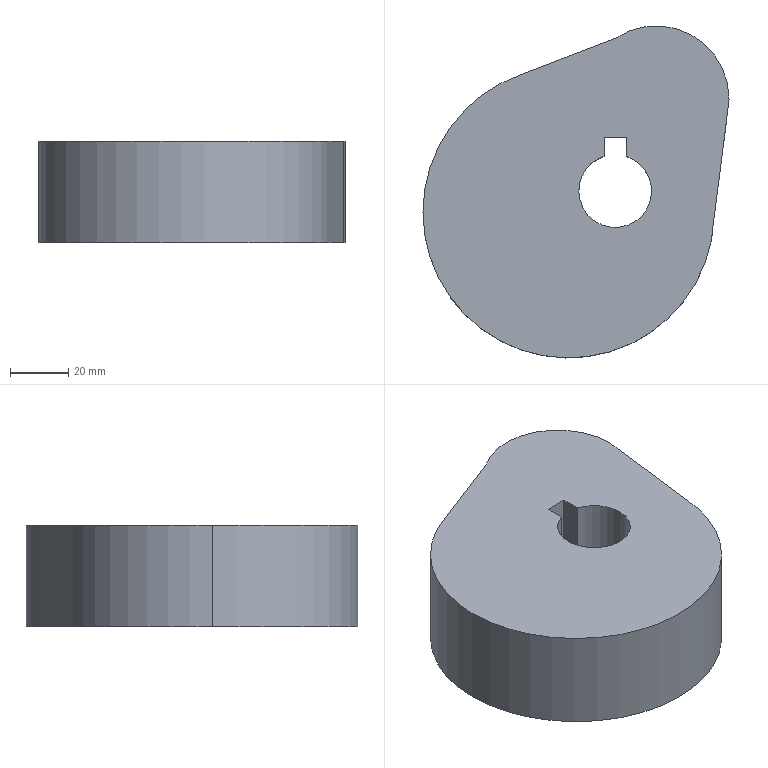Part | STEP file | Disc cam | 1 solid | 13 faces | box 105.129 x 114.018 x 35 mm | volume 298782 mm3 | plane 7 | cylinder 6 | commonest cylinder face diameters 25 x3 100 x2 50 x1
STEP:
#1=CARTESIAN_POINT('',(0.,0.,0.));
#2=DIRECTION('',(0.,0.,1.));
#3=DIRECTION('',(1.,0.,0.));
#4=AXIS2_PLACEMENT_3D('',#1,#2,#3);
#5=CARTESIAN_POINT('',(-6.022,55.403,0.));
#6=VERTEX_POINT('',#5);
#7=CARTESIAN_POINT('',(-6.022,55.403,35.));
#8=VERTEX_POINT('',#7);
#9=CARTESIAN_POINT('',(-6.022,55.403,-109.18));
#10=DIRECTION('',(0.,0.,1.));
#11=VECTOR('',#10,1.);
#12=LINE('',#9,#11);
#13=CARTESIAN_POINT('',(-18.522,55.403,-109.18));
#14=DIRECTION('',(0.,0.,1.));
#15=DIRECTION('',(1.,0.,0.));
#16=AXIS2_PLACEMENT_3D('',#13,#14,#15);
#17=CYLINDRICAL_SURFACE('',#16,12.5);
#18=CARTESIAN_POINT('',(6.283,0.));
#19=DIRECTION('',(0.,1.));
#20=VECTOR('',#19,1.);
#21=LINE('',#18,#20);
#22=(GEOMETRIC_REPRESENTATION_CONTEXT(2)PARAMETRIC_REPRESENTATION_CONTEXT()REPRESENTATION_CONTEXT('',''));
#23=DEFINITIONAL_REPRESENTATION('',(#21),#22);
#24=PCURVE('',#17,#23);
#25=CARTESIAN_POINT('',(-18.522,55.403,-109.18));
#26=DIRECTION('',(0.,0.,1.));
#27=DIRECTION('',(1.,0.,0.));
#28=AXIS2_PLACEMENT_3D('',#25,#26,#27);
#29=CYLINDRICAL_SURFACE('',#28,12.5);
#30=CARTESIAN_POINT('',(0.,0.));
#31=DIRECTION('',(0.,1.));
#32=VECTOR('',#31,1.);
#33=LINE('',#30,#32);
#34=(GEOMETRIC_REPRESENTATION_CONTEXT(2)PARAMETRIC_REPRESENTATION_CONTEXT()REPRESENTATION_CONTEXT('',''));
#35=DEFINITIONAL_REPRESENTATION('',(#33),#34);
#36=PCURVE('',#29,#35);
#37=SURFACE_CURVE('',#12,(#24,#36),.PCURVE_S1.);
#38=EDGE_CURVE('',#6,#8,#37,.T.);
#39=ORIENTED_EDGE('',*,*,#38,.T.);
#40=CARTESIAN_POINT('',(-31.022,55.403,35.));
#41=VERTEX_POINT('',#40);
#42=CARTESIAN_POINT('',(-18.522,55.403,35.));
#43=DIRECTION('',(0.,0.,1.));
#44=DIRECTION('',(1.,0.,0.));
#45=AXIS2_PLACEMENT_3D('',#42,#43,#44);
#46=CIRCLE('',#45,12.5);
#47=CARTESIAN_POINT('',(0.,144.18));
#48=DIRECTION('',(1.,0.));
#49=VECTOR('',#48,1.);
#50=LINE('',#47,#49);
#51=(GEOMETRIC_REPRESENTATION_CONTEXT(2)PARAMETRIC_REPRESENTATION_CONTEXT()REPRESENTATION_CONTEXT('',''));
#52=DEFINITIONAL_REPRESENTATION('',(#50),#51);
#53=PCURVE('',#17,#52);
#54=CARTESIAN_POINT('',(-34.555,48.107,35.));
#55=DIRECTION('',(0.,0.,1.));
#56=DIRECTION('',(1.,0.,0.));
#57=AXIS2_PLACEMENT_3D('',#54,#55,#56);
#58=PLANE('',#57);
#59=CARTESIAN_POINT('',(16.033,7.296));
#60=DIRECTION('',(1.,0.));
#61=AXIS2_PLACEMENT_2D('',#59,#60);
#62=CIRCLE('',#61,12.5);
#63=(GEOMETRIC_REPRESENTATION_CONTEXT(2)PARAMETRIC_REPRESENTATION_CONTEXT()REPRESENTATION_CONTEXT('',''));
#64=DEFINITIONAL_REPRESENTATION('',(#62),#63);
#65=PCURVE('',#58,#64);
#66=SURFACE_CURVE('',#46,(#53,#65),.PCURVE_S1.);
#67=EDGE_CURVE('',#41,#8,#66,.T.);
#68=ORIENTED_EDGE('',*,*,#67,.F.);
#69=CARTESIAN_POINT('',(-31.022,55.403,0.));
#70=VERTEX_POINT('',#69);
#71=CARTESIAN_POINT('',(-31.022,55.403,-109.18));
#72=DIRECTION('',(0.,0.,1.));
#73=VECTOR('',#72,1.);
#74=LINE('',#71,#73);
#75=CARTESIAN_POINT('',(3.142,0.));
#76=DIRECTION('',(0.,1.));
#77=VECTOR('',#76,1.);
#78=LINE('',#75,#77);
#79=(GEOMETRIC_REPRESENTATION_CONTEXT(2)PARAMETRIC_REPRESENTATION_CONTEXT()REPRESENTATION_CONTEXT('',''));
#80=DEFINITIONAL_REPRESENTATION('',(#78),#79);
#81=PCURVE('',#17,#80);
#82=CARTESIAN_POINT('',(-18.522,55.403,-109.18));
#83=DIRECTION('',(0.,0.,1.));
#84=DIRECTION('',(1.,0.,0.));
#85=AXIS2_PLACEMENT_3D('',#82,#83,#84);
#86=CYLINDRICAL_SURFACE('',#85,12.5);
#87=CARTESIAN_POINT('',(3.142,0.));
#88=DIRECTION('',(0.,1.));
#89=VECTOR('',#88,1.);
#90=LINE('',#87,#89);
#91=(GEOMETRIC_REPRESENTATION_CONTEXT(2)PARAMETRIC_REPRESENTATION_CONTEXT()REPRESENTATION_CONTEXT('',''));
#92=DEFINITIONAL_REPRESENTATION('',(#90),#91);
#93=PCURVE('',#86,#92);
#94=SURFACE_CURVE('',#74,(#81,#93),.PCURVE_S1.);
#95=EDGE_CURVE('',#70,#41,#94,.T.);
#96=ORIENTED_EDGE('',*,*,#95,.F.);
#97=CARTESIAN_POINT('',(-18.522,55.403,0.));
#98=DIRECTION('',(0.,0.,1.));
#99=DIRECTION('',(1.,0.,0.));
#100=AXIS2_PLACEMENT_3D('',#97,#98,#99);
#101=CIRCLE('',#100,12.5);
#102=CARTESIAN_POINT('',(0.,109.18));
#103=DIRECTION('',(1.,0.));
#104=VECTOR('',#103,1.);
#105=LINE('',#102,#104);
#106=(GEOMETRIC_REPRESENTATION_CONTEXT(2)PARAMETRIC_REPRESENTATION_CONTEXT()REPRESENTATION_CONTEXT('',''));
#107=DEFINITIONAL_REPRESENTATION('',(#105),#106);
#108=PCURVE('',#17,#107);
#109=CARTESIAN_POINT('',(-34.555,48.107,0.));
#110=DIRECTION('',(0.,0.,1.));
#111=DIRECTION('',(1.,0.,0.));
#112=AXIS2_PLACEMENT_3D('',#109,#110,#111);
#113=PLANE('',#112);
#114=CARTESIAN_POINT('',(16.033,7.296));
#115=DIRECTION('',(1.,0.));
#116=AXIS2_PLACEMENT_2D('',#114,#115);
#117=CIRCLE('',#116,12.5);
#118=(GEOMETRIC_REPRESENTATION_CONTEXT(2)PARAMETRIC_REPRESENTATION_CONTEXT()REPRESENTATION_CONTEXT('',''));
#119=DEFINITIONAL_REPRESENTATION('',(#117),#118);
#120=PCURVE('',#113,#119);
#121=SURFACE_CURVE('',#101,(#108,#120),.PCURVE_S1.);
#122=EDGE_CURVE('',#70,#6,#121,.T.);
#123=ORIENTED_EDGE('',*,*,#122,.T.);
#124=EDGE_LOOP('',(#39,#68,#96,#123));
#125=FACE_BOUND('',#124,.F.);
#126=ADVANCED_FACE('',(#125),#17,.F.);
#127=CARTESIAN_POINT('',(-14.611,67.276,0.));
#128=VERTEX_POINT('',#127);
#129=CARTESIAN_POINT('',(-14.611,67.276,35.));
#130=VERTEX_POINT('',#129);
#131=CARTESIAN_POINT('',(-14.611,67.276,-109.18));
#132=DIRECTION('',(0.,0.,1.));
#133=VECTOR('',#132,1.);
#134=LINE('',#131,#133);
#135=CARTESIAN_POINT('',(1.253,0.));
#136=DIRECTION('',(0.,1.));
#137=VECTOR('',#136,1.);
#138=LINE('',#135,#137);
#139=(GEOMETRIC_REPRESENTATION_CONTEXT(2)PARAMETRIC_REPRESENTATION_CONTEXT()REPRESENTATION_CONTEXT('',''));
#140=DEFINITIONAL_REPRESENTATION('',(#138),#139);
#141=PCURVE('',#29,#140);
#142=CARTESIAN_POINT('',(-14.678,73.903,-109.18));
#143=DIRECTION('',(0.9999,0.01005,0.));
#144=DIRECTION('',(-0.01005,0.9999,0.));
#145=AXIS2_PLACEMENT_3D('',#142,#143,#144);
#146=PLANE('',#145);
#147=CARTESIAN_POINT('',(-6.628,0.));
#148=DIRECTION('',(0.,1.));
#149=VECTOR('',#148,1.);
#150=LINE('',#147,#149);
#151=(GEOMETRIC_REPRESENTATION_CONTEXT(2)PARAMETRIC_REPRESENTATION_CONTEXT()REPRESENTATION_CONTEXT('',''));
#152=DEFINITIONAL_REPRESENTATION('',(#150),#151);
#153=PCURVE('',#146,#152);
#154=SURFACE_CURVE('',#134,(#141,#153),.PCURVE_S1.);
#155=EDGE_CURVE('',#128,#130,#154,.T.);
#156=ORIENTED_EDGE('',*,*,#155,.T.);
#157=CARTESIAN_POINT('',(-18.522,55.403,35.));
#158=DIRECTION('',(0.,0.,1.));
#159=DIRECTION('',(1.,0.,0.));
#160=AXIS2_PLACEMENT_3D('',#157,#158,#159);
#161=CIRCLE('',#160,12.5);
#162=CARTESIAN_POINT('',(0.,144.18));
#163=DIRECTION('',(1.,0.));
#164=VECTOR('',#163,1.);
#165=LINE('',#162,#164);
#166=(GEOMETRIC_REPRESENTATION_CONTEXT(2)PARAMETRIC_REPRESENTATION_CONTEXT()REPRESENTATION_CONTEXT('',''));
#167=DEFINITIONAL_REPRESENTATION('',(#165),#166);
#168=PCURVE('',#29,#167);
#169=CARTESIAN_POINT('',(16.033,7.296));
#170=DIRECTION('',(1.,0.));
#171=AXIS2_PLACEMENT_2D('',#169,#170);
#172=CIRCLE('',#171,12.5);
#173=(GEOMETRIC_REPRESENTATION_CONTEXT(2)PARAMETRIC_REPRESENTATION_CONTEXT()REPRESENTATION_CONTEXT('',''));
#174=DEFINITIONAL_REPRESENTATION('',(#172),#173);
#175=PCURVE('',#58,#174);
#176=SURFACE_CURVE('',#161,(#168,#175),.PCURVE_S1.);
#177=EDGE_CURVE('',#8,#130,#176,.T.);
#178=ORIENTED_EDGE('',*,*,#177,.F.);
#179=ORIENTED_EDGE('',*,*,#38,.F.);
#180=CARTESIAN_POINT('',(-18.522,55.403,0.));
#181=DIRECTION('',(0.,0.,1.));
#182=DIRECTION('',(1.,0.,0.));
#183=AXIS2_PLACEMENT_3D('',#180,#181,#182);
#184=CIRCLE('',#183,12.5);
#185=CARTESIAN_POINT('',(0.,109.18));
#186=DIRECTION('',(1.,0.));
#187=VECTOR('',#186,1.);
#188=LINE('',#185,#187);
#189=(GEOMETRIC_REPRESENTATION_CONTEXT(2)PARAMETRIC_REPRESENTATION_CONTEXT()REPRESENTATION_CONTEXT('',''));
#190=DEFINITIONAL_REPRESENTATION('',(#188),#189);
#191=PCURVE('',#29,#190);
#192=CARTESIAN_POINT('',(16.033,7.296));
#193=DIRECTION('',(1.,0.));
#194=AXIS2_PLACEMENT_2D('',#192,#193);
#195=CIRCLE('',#194,12.5);
#196=(GEOMETRIC_REPRESENTATION_CONTEXT(2)PARAMETRIC_REPRESENTATION_CONTEXT()REPRESENTATION_CONTEXT('',''));
#197=DEFINITIONAL_REPRESENTATION('',(#195),#196);
#198=PCURVE('',#113,#197);
#199=SURFACE_CURVE('',#184,(#191,#198),.PCURVE_S1.);
#200=EDGE_CURVE('',#6,#128,#199,.T.);
#201=ORIENTED_EDGE('',*,*,#200,.T.);
#202=EDGE_LOOP('',(#156,#178,#179,#201));
#203=FACE_BOUND('',#202,.F.);
#204=ADVANCED_FACE('',(#203),#29,.F.);
#205=CARTESIAN_POINT('',(-84.555,48.107,35.));
#206=VERTEX_POINT('',#205);
#207=CARTESIAN_POINT('',(15.398,45.94,35.));
#208=VERTEX_POINT('',#207);
#209=CARTESIAN_POINT('',(-34.555,48.107,35.));
#210=DIRECTION('',(0.,0.,1.));
#211=DIRECTION('',(1.,0.,0.));
#212=AXIS2_PLACEMENT_3D('',#209,#210,#211);
#213=CIRCLE('',#212,50.);
#214=CARTESIAN_POINT('',(-34.555,48.107,35.));
#215=DIRECTION('',(0.,0.,-1.));
#216=DIRECTION('',(-1.,0.,0.));
#217=AXIS2_PLACEMENT_3D('',#214,#215,#216);
#218=CYLINDRICAL_SURFACE('',#217,50.);
#219=CARTESIAN_POINT('',(9.425,0.));
#220=DIRECTION('',(-1.,0.));
#221=VECTOR('',#220,1.);
#222=LINE('',#219,#221);
#223=(GEOMETRIC_REPRESENTATION_CONTEXT(2)PARAMETRIC_REPRESENTATION_CONTEXT()REPRESENTATION_CONTEXT('',''));
#224=DEFINITIONAL_REPRESENTATION('',(#222),#223);
#225=PCURVE('',#218,#224);
#226=CARTESIAN_POINT('',(0.,0.));
#227=DIRECTION('',(1.,0.));
#228=AXIS2_PLACEMENT_2D('',#226,#227);
#229=CIRCLE('',#228,50.);
#230=(GEOMETRIC_REPRESENTATION_CONTEXT(2)PARAMETRIC_REPRESENTATION_CONTEXT()REPRESENTATION_CONTEXT('',''));
#231=DEFINITIONAL_REPRESENTATION('',(#229),#230);
#232=PCURVE('',#58,#231);
#233=SURFACE_CURVE('',#213,(#225,#232),.PCURVE_S1.);
#234=EDGE_CURVE('',#206,#208,#233,.T.);
#235=ORIENTED_EDGE('',*,*,#234,.F.);
#236=CARTESIAN_POINT('',(-84.555,48.107,0.));
#237=VERTEX_POINT('',#236);
#238=CARTESIAN_POINT('',(-84.555,48.107,35.));
#239=DIRECTION('',(0.,0.,-1.));
#240=VECTOR('',#239,1.);
#241=LINE('',#238,#240);
#242=CARTESIAN_POINT('',(6.283,0.));
#243=DIRECTION('',(0.,1.));
#244=VECTOR('',#243,1.);
#245=LINE('',#242,#244);
#246=(GEOMETRIC_REPRESENTATION_CONTEXT(2)PARAMETRIC_REPRESENTATION_CONTEXT()REPRESENTATION_CONTEXT('',''));
#247=DEFINITIONAL_REPRESENTATION('',(#245),#246);
#248=PCURVE('',#218,#247);
#249=CARTESIAN_POINT('',(-34.555,48.107,35.));
#250=DIRECTION('',(0.,0.,-1.));
#251=DIRECTION('',(-1.,0.,0.));
#252=AXIS2_PLACEMENT_3D('',#249,#250,#251);
#253=CYLINDRICAL_SURFACE('',#252,50.);
#254=CARTESIAN_POINT('',(0.,0.));
#255=DIRECTION('',(0.,1.));
#256=VECTOR('',#255,1.);
#257=LINE('',#254,#256);
#258=(GEOMETRIC_REPRESENTATION_CONTEXT(2)PARAMETRIC_REPRESENTATION_CONTEXT()REPRESENTATION_CONTEXT('',''));
#259=DEFINITIONAL_REPRESENTATION('',(#257),#258);
#260=PCURVE('',#253,#259);
#261=SURFACE_CURVE('',#241,(#248,#260),.PCURVE_S1.);
#262=EDGE_CURVE('',#206,#237,#261,.T.);
#263=ORIENTED_EDGE('',*,*,#262,.T.);
#264=CARTESIAN_POINT('',(15.398,45.94,0.));
#265=VERTEX_POINT('',#264);
#266=CARTESIAN_POINT('',(-34.555,48.107,0.));
#267=DIRECTION('',(0.,0.,1.));
#268=DIRECTION('',(1.,0.,0.));
#269=AXIS2_PLACEMENT_3D('',#266,#267,#268);
#270=CIRCLE('',#269,50.);
#271=CARTESIAN_POINT('',(9.425,35.));
#272=DIRECTION('',(-1.,0.));
#273=VECTOR('',#272,1.);
#274=LINE('',#271,#273);
#275=(GEOMETRIC_REPRESENTATION_CONTEXT(2)PARAMETRIC_REPRESENTATION_CONTEXT()REPRESENTATION_CONTEXT('',''));
#276=DEFINITIONAL_REPRESENTATION('',(#274),#275);
#277=PCURVE('',#218,#276);
#278=CARTESIAN_POINT('',(0.,0.));
#279=DIRECTION('',(1.,0.));
#280=AXIS2_PLACEMENT_2D('',#278,#279);
#281=CIRCLE('',#280,50.);
#282=(GEOMETRIC_REPRESENTATION_CONTEXT(2)PARAMETRIC_REPRESENTATION_CONTEXT()REPRESENTATION_CONTEXT('',''));
#283=DEFINITIONAL_REPRESENTATION('',(#281),#282);
#284=PCURVE('',#113,#283);
#285=SURFACE_CURVE('',#270,(#277,#284),.PCURVE_S1.);
#286=EDGE_CURVE('',#237,#265,#285,.T.);
#287=ORIENTED_EDGE('',*,*,#286,.T.);
#288=CARTESIAN_POINT('',(15.398,45.94,35.));
#289=DIRECTION('',(0.,0.,-1.));
#290=VECTOR('',#289,1.);
#291=LINE('',#288,#290);
#292=CARTESIAN_POINT('',(3.185,0.));
#293=DIRECTION('',(0.,1.));
#294=VECTOR('',#293,1.);
#295=LINE('',#292,#294);
#296=(GEOMETRIC_REPRESENTATION_CONTEXT(2)PARAMETRIC_REPRESENTATION_CONTEXT()REPRESENTATION_CONTEXT('',''));
#297=DEFINITIONAL_REPRESENTATION('',(#295),#296);
#298=PCURVE('',#218,#297);
#299=CARTESIAN_POINT('',(19.954,81.591,35.));
#300=DIRECTION('',(-0.9919,0.1268,0.));
#301=DIRECTION('',(-0.1268,-0.9919,0.));
#302=AXIS2_PLACEMENT_3D('',#299,#300,#301);
#303=PLANE('',#302);
#304=CARTESIAN_POINT('',(35.941,0.));
#305=DIRECTION('',(0.,-1.));
#306=VECTOR('',#305,1.);
#307=LINE('',#304,#306);
#308=(GEOMETRIC_REPRESENTATION_CONTEXT(2)PARAMETRIC_REPRESENTATION_CONTEXT()REPRESENTATION_CONTEXT('',''));
#309=DEFINITIONAL_REPRESENTATION('',(#307),#308);
#310=PCURVE('',#303,#309);
#311=SURFACE_CURVE('',#291,(#298,#310),.PCURVE_S1.);
#312=EDGE_CURVE('',#208,#265,#311,.T.);
#313=ORIENTED_EDGE('',*,*,#312,.F.);
#314=EDGE_LOOP('',(#235,#263,#287,#313));
#315=FACE_BOUND('',#314,.T.);
#316=ADVANCED_FACE('',(#315),#218,.T.);
#317=ORIENTED_EDGE('',*,*,#262,.F.);
#318=CARTESIAN_POINT('',(-50.63,95.453,35.));
#319=VERTEX_POINT('',#318);
#320=CARTESIAN_POINT('',(-34.555,48.107,35.));
#321=DIRECTION('',(0.,0.,1.));
#322=DIRECTION('',(1.,0.,0.));
#323=AXIS2_PLACEMENT_3D('',#320,#321,#322);
#324=CIRCLE('',#323,50.);
#325=CARTESIAN_POINT('',(3.142,0.));
#326=DIRECTION('',(-1.,0.));
#327=VECTOR('',#326,1.);
#328=LINE('',#325,#327);
#329=(GEOMETRIC_REPRESENTATION_CONTEXT(2)PARAMETRIC_REPRESENTATION_CONTEXT()REPRESENTATION_CONTEXT('',''));
#330=DEFINITIONAL_REPRESENTATION('',(#328),#329);
#331=PCURVE('',#253,#330);
#332=CARTESIAN_POINT('',(0.,0.));
#333=DIRECTION('',(1.,0.));
#334=AXIS2_PLACEMENT_2D('',#332,#333);
#335=CIRCLE('',#334,50.);
#336=(GEOMETRIC_REPRESENTATION_CONTEXT(2)PARAMETRIC_REPRESENTATION_CONTEXT()REPRESENTATION_CONTEXT('',''));
#337=DEFINITIONAL_REPRESENTATION('',(#335),#336);
#338=PCURVE('',#58,#337);
#339=SURFACE_CURVE('',#324,(#331,#338),.PCURVE_S1.);
#340=EDGE_CURVE('',#319,#206,#339,.T.);
#341=ORIENTED_EDGE('',*,*,#340,.F.);
#342=CARTESIAN_POINT('',(-50.63,95.453,0.));
#343=VERTEX_POINT('',#342);
#344=CARTESIAN_POINT('',(-50.63,95.453,35.));
#345=DIRECTION('',(0.,0.,-1.));
#346=VECTOR('',#345,1.);
#347=LINE('',#344,#346);
#348=CARTESIAN_POINT('',(1.243,0.));
#349=DIRECTION('',(0.,1.));
#350=VECTOR('',#349,1.);
#351=LINE('',#348,#350);
#352=(GEOMETRIC_REPRESENTATION_CONTEXT(2)PARAMETRIC_REPRESENTATION_CONTEXT()REPRESENTATION_CONTEXT('',''));
#353=DEFINITIONAL_REPRESENTATION('',(#351),#352);
#354=PCURVE('',#253,#353);
#355=CARTESIAN_POINT('',(-18.332,107.901,35.));
#356=DIRECTION('',(0.3596,-0.9331,0.));
#357=DIRECTION('',(0.9331,0.3596,0.));
#358=AXIS2_PLACEMENT_3D('',#355,#356,#357);
#359=PLANE('',#358);
#360=CARTESIAN_POINT('',(-34.614,0.));
#361=DIRECTION('',(0.,-1.));
#362=VECTOR('',#361,1.);
#363=LINE('',#360,#362);
#364=(GEOMETRIC_REPRESENTATION_CONTEXT(2)PARAMETRIC_REPRESENTATION_CONTEXT()REPRESENTATION_CONTEXT('',''));
#365=DEFINITIONAL_REPRESENTATION('',(#363),#364);
#366=PCURVE('',#359,#365);
#367=SURFACE_CURVE('',#347,(#354,#366),.PCURVE_S1.);
#368=EDGE_CURVE('',#319,#343,#367,.T.);
#369=ORIENTED_EDGE('',*,*,#368,.T.);
#370=CARTESIAN_POINT('',(-34.555,48.107,0.));
#371=DIRECTION('',(0.,0.,1.));
#372=DIRECTION('',(1.,0.,0.));
#373=AXIS2_PLACEMENT_3D('',#370,#371,#372);
#374=CIRCLE('',#373,50.);
#375=CARTESIAN_POINT('',(3.142,35.));
#376=DIRECTION('',(-1.,0.));
#377=VECTOR('',#376,1.);
#378=LINE('',#375,#377);
#379=(GEOMETRIC_REPRESENTATION_CONTEXT(2)PARAMETRIC_REPRESENTATION_CONTEXT()REPRESENTATION_CONTEXT('',''));
#380=DEFINITIONAL_REPRESENTATION('',(#378),#379);
#381=PCURVE('',#253,#380);
#382=CARTESIAN_POINT('',(0.,0.));
#383=DIRECTION('',(1.,0.));
#384=AXIS2_PLACEMENT_2D('',#382,#383);
#385=CIRCLE('',#384,50.);
#386=(GEOMETRIC_REPRESENTATION_CONTEXT(2)PARAMETRIC_REPRESENTATION_CONTEXT()REPRESENTATION_CONTEXT('',''));
#387=DEFINITIONAL_REPRESENTATION('',(#385),#386);
#388=PCURVE('',#113,#387);
#389=SURFACE_CURVE('',#374,(#381,#388),.PCURVE_S1.);
#390=EDGE_CURVE('',#343,#237,#389,.T.);
#391=ORIENTED_EDGE('',*,*,#390,.T.);
#392=EDGE_LOOP('',(#317,#341,#369,#391));
#393=FACE_BOUND('',#392,.T.);
#394=ADVANCED_FACE('',(#393),#253,.T.);
#395=CARTESIAN_POINT('',(19.954,81.591,0.));
#396=VERTEX_POINT('',#395);
#397=CARTESIAN_POINT('',(19.954,81.591,0.));
#398=DIRECTION('',(0.1268,0.9919,0.));
#399=VECTOR('',#398,1.);
#400=LINE('',#397,#399);
#401=CARTESIAN_POINT('',(0.,-35.));
#402=DIRECTION('',(-1.,0.));
#403=VECTOR('',#402,1.);
#404=LINE('',#401,#403);
#405=(GEOMETRIC_REPRESENTATION_CONTEXT(2)PARAMETRIC_REPRESENTATION_CONTEXT()REPRESENTATION_CONTEXT('',''));
#406=DEFINITIONAL_REPRESENTATION('',(#404),#405);
#407=PCURVE('',#303,#406);
#408=CARTESIAN_POINT('',(54.509,33.484));
#409=DIRECTION('',(0.1268,0.9919));
#410=VECTOR('',#409,1.);
#411=LINE('',#408,#410);
#412=(GEOMETRIC_REPRESENTATION_CONTEXT(2)PARAMETRIC_REPRESENTATION_CONTEXT()REPRESENTATION_CONTEXT('',''));
#413=DEFINITIONAL_REPRESENTATION('',(#411),#412);
#414=PCURVE('',#113,#413);
#415=SURFACE_CURVE('',#400,(#407,#414),.PCURVE_S1.);
#416=EDGE_CURVE('',#265,#396,#415,.T.);
#417=ORIENTED_EDGE('',*,*,#416,.T.);
#418=CARTESIAN_POINT('',(19.954,81.591,35.));
#419=VERTEX_POINT('',#418);
#420=CARTESIAN_POINT('',(19.954,81.591,35.));
#421=DIRECTION('',(0.,0.,-1.));
#422=VECTOR('',#421,1.);
#423=LINE('',#420,#422);
#424=CARTESIAN_POINT('',(0.,0.));
#425=DIRECTION('',(0.,-1.));
#426=VECTOR('',#425,1.);
#427=LINE('',#424,#426);
#428=(GEOMETRIC_REPRESENTATION_CONTEXT(2)PARAMETRIC_REPRESENTATION_CONTEXT()REPRESENTATION_CONTEXT('',''));
#429=DEFINITIONAL_REPRESENTATION('',(#427),#428);
#430=PCURVE('',#303,#429);
#431=CARTESIAN_POINT('',(-4.426,87.125,35.));
#432=DIRECTION('',(0.,0.,-1.));
#433=DIRECTION('',(-1.,0.,0.));
#434=AXIS2_PLACEMENT_3D('',#431,#432,#433);
#435=CYLINDRICAL_SURFACE('',#434,25.);
#436=CARTESIAN_POINT('',(3.365,0.));
#437=DIRECTION('',(0.,1.));
#438=VECTOR('',#437,1.);
#439=LINE('',#436,#438);
#440=(GEOMETRIC_REPRESENTATION_CONTEXT(2)PARAMETRIC_REPRESENTATION_CONTEXT()REPRESENTATION_CONTEXT('',''));
#441=DEFINITIONAL_REPRESENTATION('',(#439),#440);
#442=PCURVE('',#435,#441);
#443=SURFACE_CURVE('',#423,(#430,#442),.PCURVE_S1.);
#444=EDGE_CURVE('',#419,#396,#443,.T.);
#445=ORIENTED_EDGE('',*,*,#444,.F.);
#446=CARTESIAN_POINT('',(19.954,81.591,35.));
#447=DIRECTION('',(0.1268,0.9919,0.));
#448=VECTOR('',#447,1.);
#449=LINE('',#446,#448);
#450=CARTESIAN_POINT('',(0.,0.));
#451=DIRECTION('',(-1.,0.));
#452=VECTOR('',#451,1.);
#453=LINE('',#450,#452);
#454=(GEOMETRIC_REPRESENTATION_CONTEXT(2)PARAMETRIC_REPRESENTATION_CONTEXT()REPRESENTATION_CONTEXT('',''));
#455=DEFINITIONAL_REPRESENTATION('',(#453),#454);
#456=PCURVE('',#303,#455);
#457=CARTESIAN_POINT('',(54.509,33.484));
#458=DIRECTION('',(0.1268,0.9919));
#459=VECTOR('',#458,1.);
#460=LINE('',#457,#459);
#461=(GEOMETRIC_REPRESENTATION_CONTEXT(2)PARAMETRIC_REPRESENTATION_CONTEXT()REPRESENTATION_CONTEXT('',''));
#462=DEFINITIONAL_REPRESENTATION('',(#460),#461);
#463=PCURVE('',#58,#462);
#464=SURFACE_CURVE('',#449,(#456,#463),.PCURVE_S1.);
#465=EDGE_CURVE('',#208,#419,#464,.T.);
#466=ORIENTED_EDGE('',*,*,#465,.F.);
#467=ORIENTED_EDGE('',*,*,#312,.T.);
#468=EDGE_LOOP('',(#417,#445,#466,#467));
#469=FACE_BOUND('',#468,.T.);
#470=ADVANCED_FACE('',(#469),#303,.F.);
#471=CARTESIAN_POINT('',(-18.332,107.901,0.));
#472=VERTEX_POINT('',#471);
#473=CARTESIAN_POINT('',(-4.426,87.125,0.));
#474=DIRECTION('',(0.,0.,1.));
#475=DIRECTION('',(1.,0.,0.));
#476=AXIS2_PLACEMENT_3D('',#473,#474,#475);
#477=CIRCLE('',#476,25.);
#478=CARTESIAN_POINT('',(9.425,35.));
#479=DIRECTION('',(-1.,0.));
#480=VECTOR('',#479,1.);
#481=LINE('',#478,#480);
#482=(GEOMETRIC_REPRESENTATION_CONTEXT(2)PARAMETRIC_REPRESENTATION_CONTEXT()REPRESENTATION_CONTEXT('',''));
#483=DEFINITIONAL_REPRESENTATION('',(#481),#482);
#484=PCURVE('',#435,#483);
#485=CARTESIAN_POINT('',(30.129,39.018));
#486=DIRECTION('',(1.,0.));
#487=AXIS2_PLACEMENT_2D('',#485,#486);
#488=CIRCLE('',#487,25.);
#489=(GEOMETRIC_REPRESENTATION_CONTEXT(2)PARAMETRIC_REPRESENTATION_CONTEXT()REPRESENTATION_CONTEXT('',''));
#490=DEFINITIONAL_REPRESENTATION('',(#488),#489);
#491=PCURVE('',#113,#490);
#492=SURFACE_CURVE('',#477,(#484,#491),.PCURVE_S1.);
#493=EDGE_CURVE('',#396,#472,#492,.T.);
#494=ORIENTED_EDGE('',*,*,#493,.T.);
#495=CARTESIAN_POINT('',(-18.332,107.901,35.));
#496=VERTEX_POINT('',#495);
#497=CARTESIAN_POINT('',(-18.332,107.901,35.));
#498=DIRECTION('',(0.,0.,-1.));
#499=VECTOR('',#498,1.);
#500=LINE('',#497,#499);
#501=CARTESIAN_POINT('',(0.981,0.));
#502=DIRECTION('',(0.,1.));
#503=VECTOR('',#502,1.);
#504=LINE('',#501,#503);
#505=(GEOMETRIC_REPRESENTATION_CONTEXT(2)PARAMETRIC_REPRESENTATION_CONTEXT()REPRESENTATION_CONTEXT('',''));
#506=DEFINITIONAL_REPRESENTATION('',(#504),#505);
#507=PCURVE('',#435,#506);
#508=CARTESIAN_POINT('',(0.,0.));
#509=DIRECTION('',(0.,-1.));
#510=VECTOR('',#509,1.);
#511=LINE('',#508,#510);
#512=(GEOMETRIC_REPRESENTATION_CONTEXT(2)PARAMETRIC_REPRESENTATION_CONTEXT()REPRESENTATION_CONTEXT('',''));
#513=DEFINITIONAL_REPRESENTATION('',(#511),#512);
#514=PCURVE('',#359,#513);
#515=SURFACE_CURVE('',#500,(#507,#514),.PCURVE_S1.);
#516=EDGE_CURVE('',#496,#472,#515,.T.);
#517=ORIENTED_EDGE('',*,*,#516,.F.);
#518=CARTESIAN_POINT('',(-4.426,87.125,35.));
#519=DIRECTION('',(0.,0.,1.));
#520=DIRECTION('',(1.,0.,0.));
#521=AXIS2_PLACEMENT_3D('',#518,#519,#520);
#522=CIRCLE('',#521,25.);
#523=CARTESIAN_POINT('',(9.425,0.));
#524=DIRECTION('',(-1.,0.));
#525=VECTOR('',#524,1.);
#526=LINE('',#523,#525);
#527=(GEOMETRIC_REPRESENTATION_CONTEXT(2)PARAMETRIC_REPRESENTATION_CONTEXT()REPRESENTATION_CONTEXT('',''));
#528=DEFINITIONAL_REPRESENTATION('',(#526),#527);
#529=PCURVE('',#435,#528);
#530=CARTESIAN_POINT('',(30.129,39.018));
#531=DIRECTION('',(1.,0.));
#532=AXIS2_PLACEMENT_2D('',#530,#531);
#533=CIRCLE('',#532,25.);
#534=(GEOMETRIC_REPRESENTATION_CONTEXT(2)PARAMETRIC_REPRESENTATION_CONTEXT()REPRESENTATION_CONTEXT('',''));
#535=DEFINITIONAL_REPRESENTATION('',(#533),#534);
#536=PCURVE('',#58,#535);
#537=SURFACE_CURVE('',#522,(#529,#536),.PCURVE_S1.);
#538=EDGE_CURVE('',#419,#496,#537,.T.);
#539=ORIENTED_EDGE('',*,*,#538,.F.);
#540=ORIENTED_EDGE('',*,*,#444,.T.);
#541=EDGE_LOOP('',(#494,#517,#539,#540));
#542=FACE_BOUND('',#541,.T.);
#543=ADVANCED_FACE('',(#542),#435,.T.);
#544=CARTESIAN_POINT('',(-18.332,107.901,0.));
#545=DIRECTION('',(-0.9331,-0.3596,0.));
#546=VECTOR('',#545,1.);
#547=LINE('',#544,#546);
#548=CARTESIAN_POINT('',(0.,-35.));
#549=DIRECTION('',(-1.,0.));
#550=VECTOR('',#549,1.);
#551=LINE('',#548,#550);
#552=(GEOMETRIC_REPRESENTATION_CONTEXT(2)PARAMETRIC_REPRESENTATION_CONTEXT()REPRESENTATION_CONTEXT('',''));
#553=DEFINITIONAL_REPRESENTATION('',(#551),#552);
#554=PCURVE('',#359,#553);
#555=CARTESIAN_POINT('',(16.224,59.794));
#556=DIRECTION('',(-0.9331,-0.3596));
#557=VECTOR('',#556,1.);
#558=LINE('',#555,#557);
#559=(GEOMETRIC_REPRESENTATION_CONTEXT(2)PARAMETRIC_REPRESENTATION_CONTEXT()REPRESENTATION_CONTEXT('',''));
#560=DEFINITIONAL_REPRESENTATION('',(#558),#559);
#561=PCURVE('',#113,#560);
#562=SURFACE_CURVE('',#547,(#554,#561),.PCURVE_S1.);
#563=EDGE_CURVE('',#472,#343,#562,.T.);
#564=ORIENTED_EDGE('',*,*,#563,.T.);
#565=ORIENTED_EDGE('',*,*,#368,.F.);
#566=CARTESIAN_POINT('',(-18.332,107.901,35.));
#567=DIRECTION('',(-0.9331,-0.3596,0.));
#568=VECTOR('',#567,1.);
#569=LINE('',#566,#568);
#570=CARTESIAN_POINT('',(0.,0.));
#571=DIRECTION('',(-1.,0.));
#572=VECTOR('',#571,1.);
#573=LINE('',#570,#572);
#574=(GEOMETRIC_REPRESENTATION_CONTEXT(2)PARAMETRIC_REPRESENTATION_CONTEXT()REPRESENTATION_CONTEXT('',''));
#575=DEFINITIONAL_REPRESENTATION('',(#573),#574);
#576=PCURVE('',#359,#575);
#577=CARTESIAN_POINT('',(16.224,59.794));
#578=DIRECTION('',(-0.9331,-0.3596));
#579=VECTOR('',#578,1.);
#580=LINE('',#577,#579);
#581=(GEOMETRIC_REPRESENTATION_CONTEXT(2)PARAMETRIC_REPRESENTATION_CONTEXT()REPRESENTATION_CONTEXT('',''));
#582=DEFINITIONAL_REPRESENTATION('',(#580),#581);
#583=PCURVE('',#58,#582);
#584=SURFACE_CURVE('',#569,(#576,#583),.PCURVE_S1.);
#585=EDGE_CURVE('',#496,#319,#584,.T.);
#586=ORIENTED_EDGE('',*,*,#585,.F.);
#587=ORIENTED_EDGE('',*,*,#516,.T.);
#588=EDGE_LOOP('',(#564,#565,#586,#587));
#589=FACE_BOUND('',#588,.T.);
#590=ADVANCED_FACE('',(#589),#359,.F.);
#591=CARTESIAN_POINT('',(-22.366,67.297,35.));
#592=VERTEX_POINT('',#591);
#593=CARTESIAN_POINT('',(-18.522,55.403,35.));
#594=DIRECTION('',(0.,0.,1.));
#595=DIRECTION('',(1.,0.,0.));
#596=AXIS2_PLACEMENT_3D('',#593,#594,#595);
#597=CIRCLE('',#596,12.5);
#598=CARTESIAN_POINT('',(16.033,7.296));
#599=DIRECTION('',(1.,0.));
#600=AXIS2_PLACEMENT_2D('',#598,#599);
#601=CIRCLE('',#600,12.5);
#602=(GEOMETRIC_REPRESENTATION_CONTEXT(2)PARAMETRIC_REPRESENTATION_CONTEXT()REPRESENTATION_CONTEXT('',''));
#603=DEFINITIONAL_REPRESENTATION('',(#601),#602);
#604=PCURVE('',#58,#603);
#605=CARTESIAN_POINT('',(0.,144.18));
#606=DIRECTION('',(1.,0.));
#607=VECTOR('',#606,1.);
#608=LINE('',#605,#607);
#609=(GEOMETRIC_REPRESENTATION_CONTEXT(2)PARAMETRIC_REPRESENTATION_CONTEXT()REPRESENTATION_CONTEXT('',''));
#610=DEFINITIONAL_REPRESENTATION('',(#608),#609);
#611=PCURVE('',#86,#610);
#612=SURFACE_CURVE('',#597,(#604,#611),.PCURVE_S1.);
#613=EDGE_CURVE('',#592,#41,#612,.T.);
#614=ORIENTED_EDGE('',*,*,#613,.F.);
#615=CARTESIAN_POINT('',(-22.366,73.903,35.));
#616=VERTEX_POINT('',#615);
#617=CARTESIAN_POINT('',(-22.366,73.903,35.));
#618=DIRECTION('',(0.,-1.,0.));
#619=VECTOR('',#618,1.);
#620=LINE('',#617,#619);
#621=CARTESIAN_POINT('',(12.189,25.796));
#622=DIRECTION('',(0.,-1.));
#623=VECTOR('',#622,1.);
#624=LINE('',#621,#623);
#625=(GEOMETRIC_REPRESENTATION_CONTEXT(2)PARAMETRIC_REPRESENTATION_CONTEXT()REPRESENTATION_CONTEXT('',''));
#626=DEFINITIONAL_REPRESENTATION('',(#624),#625);
#627=PCURVE('',#58,#626);
#628=CARTESIAN_POINT('',(-22.366,73.903,-109.18));
#629=DIRECTION('',(-1.,0.,0.));
#630=DIRECTION('',(0.,-1.,0.));
#631=AXIS2_PLACEMENT_3D('',#628,#629,#630);
#632=PLANE('',#631);
#633=CARTESIAN_POINT('',(0.,144.18));
#634=DIRECTION('',(1.,0.));
#635=VECTOR('',#634,1.);
#636=LINE('',#633,#635);
#637=(GEOMETRIC_REPRESENTATION_CONTEXT(2)PARAMETRIC_REPRESENTATION_CONTEXT()REPRESENTATION_CONTEXT('',''));
#638=DEFINITIONAL_REPRESENTATION('',(#636),#637);
#639=PCURVE('',#632,#638);
#640=SURFACE_CURVE('',#620,(#627,#639),.PCURVE_S1.);
#641=EDGE_CURVE('',#616,#592,#640,.T.);
#642=ORIENTED_EDGE('',*,*,#641,.F.);
#643=CARTESIAN_POINT('',(-14.678,73.903,35.));
#644=VERTEX_POINT('',#643);
#645=CARTESIAN_POINT('',(-22.366,73.903,35.));
#646=DIRECTION('',(-1.,0.,0.));
#647=VECTOR('',#646,1.);
#648=LINE('',#645,#647);
#649=CARTESIAN_POINT('',(12.189,25.796));
#650=DIRECTION('',(-1.,0.));
#651=VECTOR('',#650,1.);
#652=LINE('',#649,#651);
#653=(GEOMETRIC_REPRESENTATION_CONTEXT(2)PARAMETRIC_REPRESENTATION_CONTEXT()REPRESENTATION_CONTEXT('',''));
#654=DEFINITIONAL_REPRESENTATION('',(#652),#653);
#655=PCURVE('',#58,#654);
#656=CARTESIAN_POINT('',(-22.366,73.903,-109.18));
#657=DIRECTION('',(0.,1.,0.));
#658=DIRECTION('',(0.,0.,1.));
#659=AXIS2_PLACEMENT_3D('',#656,#657,#658);
#660=PLANE('',#659);
#661=CARTESIAN_POINT('',(144.18,0.));
#662=DIRECTION('',(0.,-1.));
#663=VECTOR('',#662,1.);
#664=LINE('',#661,#663);
#665=(GEOMETRIC_REPRESENTATION_CONTEXT(2)PARAMETRIC_REPRESENTATION_CONTEXT()REPRESENTATION_CONTEXT('',''));
#666=DEFINITIONAL_REPRESENTATION('',(#664),#665);
#667=PCURVE('',#660,#666);
#668=SURFACE_CURVE('',#648,(#655,#667),.PCURVE_S1.);
#669=EDGE_CURVE('',#644,#616,#668,.T.);
#670=ORIENTED_EDGE('',*,*,#669,.F.);
#671=CARTESIAN_POINT('',(-14.678,73.903,35.));
#672=DIRECTION('',(-0.01005,0.9999,0.));
#673=VECTOR('',#672,1.);
#674=LINE('',#671,#673);
#675=CARTESIAN_POINT('',(19.878,25.796));
#676=DIRECTION('',(-0.01005,0.9999));
#677=VECTOR('',#676,1.);
#678=LINE('',#675,#677);
#679=(GEOMETRIC_REPRESENTATION_CONTEXT(2)PARAMETRIC_REPRESENTATION_CONTEXT()REPRESENTATION_CONTEXT('',''));
#680=DEFINITIONAL_REPRESENTATION('',(#678),#679);
#681=PCURVE('',#58,#680);
#682=CARTESIAN_POINT('',(0.,144.18));
#683=DIRECTION('',(1.,0.));
#684=VECTOR('',#683,1.);
#685=LINE('',#682,#684);
#686=(GEOMETRIC_REPRESENTATION_CONTEXT(2)PARAMETRIC_REPRESENTATION_CONTEXT()REPRESENTATION_CONTEXT('',''));
#687=DEFINITIONAL_REPRESENTATION('',(#685),#686);
#688=PCURVE('',#146,#687);
#689=SURFACE_CURVE('',#674,(#681,#688),.PCURVE_S1.);
#690=EDGE_CURVE('',#130,#644,#689,.T.);
#691=ORIENTED_EDGE('',*,*,#690,.F.);
#692=ORIENTED_EDGE('',*,*,#177,.F.);
#693=ORIENTED_EDGE('',*,*,#67,.F.);
#694=EDGE_LOOP('',(#614,#642,#670,#691,#692,#693));
#695=FACE_BOUND('',#694,.T.);
#696=ORIENTED_EDGE('',*,*,#340,.T.);
#697=ORIENTED_EDGE('',*,*,#234,.T.);
#698=ORIENTED_EDGE('',*,*,#465,.T.);
#699=ORIENTED_EDGE('',*,*,#538,.T.);
#700=ORIENTED_EDGE('',*,*,#585,.T.);
#701=EDGE_LOOP('',(#696,#697,#698,#699,#700));
#702=FACE_BOUND('',#701,.T.);
#703=ADVANCED_FACE('',(#695,#702),#58,.T.);
#704=CARTESIAN_POINT('',(-22.366,73.903,0.));
#705=VERTEX_POINT('',#704);
#706=CARTESIAN_POINT('',(-22.366,67.297,0.));
#707=VERTEX_POINT('',#706);
#708=CARTESIAN_POINT('',(-22.366,48.107,0.));
#709=DIRECTION('',(0.,-1.,0.));
#710=VECTOR('',#709,1.);
#711=LINE('',#708,#710);
#712=CARTESIAN_POINT('',(12.189,0.));
#713=DIRECTION('',(0.,-1.));
#714=VECTOR('',#713,1.);
#715=LINE('',#712,#714);
#716=(GEOMETRIC_REPRESENTATION_CONTEXT(2)PARAMETRIC_REPRESENTATION_CONTEXT()REPRESENTATION_CONTEXT('',''));
#717=DEFINITIONAL_REPRESENTATION('',(#715),#716);
#718=PCURVE('',#113,#717);
#719=CARTESIAN_POINT('',(25.796,109.18));
#720=DIRECTION('',(1.,0.));
#721=VECTOR('',#720,1.);
#722=LINE('',#719,#721);
#723=(GEOMETRIC_REPRESENTATION_CONTEXT(2)PARAMETRIC_REPRESENTATION_CONTEXT()REPRESENTATION_CONTEXT('',''));
#724=DEFINITIONAL_REPRESENTATION('',(#722),#723);
#725=PCURVE('',#632,#724);
#726=SURFACE_CURVE('',#711,(#718,#725),.PCURVE_S1.);
#727=EDGE_CURVE('',#705,#707,#726,.T.);
#728=ORIENTED_EDGE('',*,*,#727,.T.);
#729=CARTESIAN_POINT('',(-18.522,55.403,0.));
#730=DIRECTION('',(0.,0.,1.));
#731=DIRECTION('',(1.,0.,0.));
#732=AXIS2_PLACEMENT_3D('',#729,#730,#731);
#733=CIRCLE('',#732,12.5);
#734=CARTESIAN_POINT('',(16.033,7.296));
#735=DIRECTION('',(1.,0.));
#736=AXIS2_PLACEMENT_2D('',#734,#735);
#737=CIRCLE('',#736,12.5);
#738=(GEOMETRIC_REPRESENTATION_CONTEXT(2)PARAMETRIC_REPRESENTATION_CONTEXT()REPRESENTATION_CONTEXT('',''));
#739=DEFINITIONAL_REPRESENTATION('',(#737),#738);
#740=PCURVE('',#113,#739);
#741=CARTESIAN_POINT('',(0.,109.18));
#742=DIRECTION('',(1.,0.));
#743=VECTOR('',#742,1.);
#744=LINE('',#741,#743);
#745=(GEOMETRIC_REPRESENTATION_CONTEXT(2)PARAMETRIC_REPRESENTATION_CONTEXT()REPRESENTATION_CONTEXT('',''));
#746=DEFINITIONAL_REPRESENTATION('',(#744),#745);
#747=PCURVE('',#86,#746);
#748=SURFACE_CURVE('',#733,(#740,#747),.PCURVE_S1.);
#749=EDGE_CURVE('',#707,#70,#748,.T.);
#750=ORIENTED_EDGE('',*,*,#749,.T.);
#751=ORIENTED_EDGE('',*,*,#122,.T.);
#752=ORIENTED_EDGE('',*,*,#200,.T.);
#753=CARTESIAN_POINT('',(-14.678,73.903,0.));
#754=VERTEX_POINT('',#753);
#755=CARTESIAN_POINT('',(-14.42,48.309,0.));
#756=DIRECTION('',(-0.01005,0.9999,0.));
#757=VECTOR('',#756,1.);
#758=LINE('',#755,#757);
#759=CARTESIAN_POINT('',(20.135,0.2024));
#760=DIRECTION('',(-0.01005,0.9999));
#761=VECTOR('',#760,1.);
#762=LINE('',#759,#761);
#763=(GEOMETRIC_REPRESENTATION_CONTEXT(2)PARAMETRIC_REPRESENTATION_CONTEXT()REPRESENTATION_CONTEXT('',''));
#764=DEFINITIONAL_REPRESENTATION('',(#762),#763);
#765=PCURVE('',#113,#764);
#766=CARTESIAN_POINT('',(-25.595,109.18));
#767=DIRECTION('',(1.,0.));
#768=VECTOR('',#767,1.);
#769=LINE('',#766,#768);
#770=(GEOMETRIC_REPRESENTATION_CONTEXT(2)PARAMETRIC_REPRESENTATION_CONTEXT()REPRESENTATION_CONTEXT('',''));
#771=DEFINITIONAL_REPRESENTATION('',(#769),#770);
#772=PCURVE('',#146,#771);
#773=SURFACE_CURVE('',#758,(#765,#772),.PCURVE_S1.);
#774=EDGE_CURVE('',#128,#754,#773,.T.);
#775=ORIENTED_EDGE('',*,*,#774,.T.);
#776=CARTESIAN_POINT('',(-34.555,73.903,0.));
#777=DIRECTION('',(-1.,0.,0.));
#778=VECTOR('',#777,1.);
#779=LINE('',#776,#778);
#780=CARTESIAN_POINT('',(0.,25.796));
#781=DIRECTION('',(-1.,0.));
#782=VECTOR('',#781,1.);
#783=LINE('',#780,#782);
#784=(GEOMETRIC_REPRESENTATION_CONTEXT(2)PARAMETRIC_REPRESENTATION_CONTEXT()REPRESENTATION_CONTEXT('',''));
#785=DEFINITIONAL_REPRESENTATION('',(#783),#784);
#786=PCURVE('',#113,#785);
#787=CARTESIAN_POINT('',(109.18,-12.189));
#788=DIRECTION('',(0.,-1.));
#789=VECTOR('',#788,1.);
#790=LINE('',#787,#789);
#791=(GEOMETRIC_REPRESENTATION_CONTEXT(2)PARAMETRIC_REPRESENTATION_CONTEXT()REPRESENTATION_CONTEXT('',''));
#792=DEFINITIONAL_REPRESENTATION('',(#790),#791);
#793=PCURVE('',#660,#792);
#794=SURFACE_CURVE('',#779,(#786,#793),.PCURVE_S1.);
#795=EDGE_CURVE('',#754,#705,#794,.T.);
#796=ORIENTED_EDGE('',*,*,#795,.T.);
#797=EDGE_LOOP('',(#728,#750,#751,#752,#775,#796));
#798=FACE_BOUND('',#797,.T.);
#799=ORIENTED_EDGE('',*,*,#390,.F.);
#800=ORIENTED_EDGE('',*,*,#563,.F.);
#801=ORIENTED_EDGE('',*,*,#493,.F.);
#802=ORIENTED_EDGE('',*,*,#416,.F.);
#803=ORIENTED_EDGE('',*,*,#286,.F.);
#804=EDGE_LOOP('',(#799,#800,#801,#802,#803));
#805=FACE_BOUND('',#804,.T.);
#806=ADVANCED_FACE('',(#798,#805),#113,.F.);
#807=ORIENTED_EDGE('',*,*,#613,.F.);
#808=CARTESIAN_POINT('',(-22.366,67.297,-109.18));
#809=DIRECTION('',(0.,0.,1.));
#810=VECTOR('',#809,1.);
#811=LINE('',#808,#810);
#812=CARTESIAN_POINT('',(1.883,0.));
#813=DIRECTION('',(0.,1.));
#814=VECTOR('',#813,1.);
#815=LINE('',#812,#814);
#816=(GEOMETRIC_REPRESENTATION_CONTEXT(2)PARAMETRIC_REPRESENTATION_CONTEXT()REPRESENTATION_CONTEXT('',''));
#817=DEFINITIONAL_REPRESENTATION('',(#815),#816);
#818=PCURVE('',#86,#817);
#819=CARTESIAN_POINT('',(6.606,0.));
#820=DIRECTION('',(0.,1.));
#821=VECTOR('',#820,1.);
#822=LINE('',#819,#821);
#823=(GEOMETRIC_REPRESENTATION_CONTEXT(2)PARAMETRIC_REPRESENTATION_CONTEXT()REPRESENTATION_CONTEXT('',''));
#824=DEFINITIONAL_REPRESENTATION('',(#822),#823);
#825=PCURVE('',#632,#824);
#826=SURFACE_CURVE('',#811,(#818,#825),.PCURVE_S1.);
#827=EDGE_CURVE('',#707,#592,#826,.T.);
#828=ORIENTED_EDGE('',*,*,#827,.F.);
#829=ORIENTED_EDGE('',*,*,#749,.T.);
#830=ORIENTED_EDGE('',*,*,#95,.T.);
#831=EDGE_LOOP('',(#807,#828,#829,#830));
#832=FACE_BOUND('',#831,.F.);
#833=ADVANCED_FACE('',(#832),#86,.F.);
#834=CARTESIAN_POINT('',(-22.366,73.903,-109.18));
#835=DIRECTION('',(0.,0.,1.));
#836=VECTOR('',#835,1.);
#837=LINE('',#834,#836);
#838=CARTESIAN_POINT('',(0.,0.));
#839=DIRECTION('',(0.,1.));
#840=VECTOR('',#839,1.);
#841=LINE('',#838,#840);
#842=(GEOMETRIC_REPRESENTATION_CONTEXT(2)PARAMETRIC_REPRESENTATION_CONTEXT()REPRESENTATION_CONTEXT('',''));
#843=DEFINITIONAL_REPRESENTATION('',(#841),#842);
#844=PCURVE('',#632,#843);
#845=CARTESIAN_POINT('',(0.,0.));
#846=DIRECTION('',(1.,0.));
#847=VECTOR('',#846,1.);
#848=LINE('',#845,#847);
#849=(GEOMETRIC_REPRESENTATION_CONTEXT(2)PARAMETRIC_REPRESENTATION_CONTEXT()REPRESENTATION_CONTEXT('',''));
#850=DEFINITIONAL_REPRESENTATION('',(#848),#849);
#851=PCURVE('',#660,#850);
#852=SURFACE_CURVE('',#837,(#844,#851),.PCURVE_S1.);
#853=EDGE_CURVE('',#705,#616,#852,.T.);
#854=ORIENTED_EDGE('',*,*,#853,.T.);
#855=ORIENTED_EDGE('',*,*,#641,.T.);
#856=ORIENTED_EDGE('',*,*,#827,.F.);
#857=ORIENTED_EDGE('',*,*,#727,.F.);
#858=EDGE_LOOP('',(#854,#855,#856,#857));
#859=FACE_BOUND('',#858,.T.);
#860=ADVANCED_FACE('',(#859),#632,.F.);
#861=CARTESIAN_POINT('',(-14.678,73.903,-109.18));
#862=DIRECTION('',(0.,0.,1.));
#863=VECTOR('',#862,1.);
#864=LINE('',#861,#863);
#865=CARTESIAN_POINT('',(0.,7.689));
#866=DIRECTION('',(1.,0.));
#867=VECTOR('',#866,1.);
#868=LINE('',#865,#867);
#869=(GEOMETRIC_REPRESENTATION_CONTEXT(2)PARAMETRIC_REPRESENTATION_CONTEXT()REPRESENTATION_CONTEXT('',''));
#870=DEFINITIONAL_REPRESENTATION('',(#868),#869);
#871=PCURVE('',#660,#870);
#872=CARTESIAN_POINT('',(0.,0.));
#873=DIRECTION('',(0.,1.));
#874=VECTOR('',#873,1.);
#875=LINE('',#872,#874);
#876=(GEOMETRIC_REPRESENTATION_CONTEXT(2)PARAMETRIC_REPRESENTATION_CONTEXT()REPRESENTATION_CONTEXT('',''));
#877=DEFINITIONAL_REPRESENTATION('',(#875),#876);
#878=PCURVE('',#146,#877);
#879=SURFACE_CURVE('',#864,(#871,#878),.PCURVE_S1.);
#880=EDGE_CURVE('',#754,#644,#879,.T.);
#881=ORIENTED_EDGE('',*,*,#880,.T.);
#882=ORIENTED_EDGE('',*,*,#669,.T.);
#883=ORIENTED_EDGE('',*,*,#853,.F.);
#884=ORIENTED_EDGE('',*,*,#795,.F.);
#885=EDGE_LOOP('',(#881,#882,#883,#884));
#886=FACE_BOUND('',#885,.T.);
#887=ADVANCED_FACE('',(#886),#660,.F.);
#888=ORIENTED_EDGE('',*,*,#155,.T.);
#889=ORIENTED_EDGE('',*,*,#690,.T.);
#890=ORIENTED_EDGE('',*,*,#880,.F.);
#891=ORIENTED_EDGE('',*,*,#774,.F.);
#892=EDGE_LOOP('',(#888,#889,#890,#891));
#893=FACE_BOUND('',#892,.T.);
#894=ADVANCED_FACE('',(#893),#146,.F.);
#895=CLOSED_SHELL('',(#126,#204,#316,#394,#470,#543,#590,#703,#806,#833,#860,#887,#894));
#896=MANIFOLD_SOLID_BREP('',#895);
#897=(LENGTH_UNIT()NAMED_UNIT(*)SI_UNIT(.MILLI.,.METRE.));
#898=UNCERTAINTY_MEASURE_WITH_UNIT(LENGTH_MEASURE(0.0000001),#897,'','');
#899=(NAMED_UNIT(*)PLANE_ANGLE_UNIT()SI_UNIT($,.RADIAN.));
#900=(NAMED_UNIT(*)SI_UNIT($,.STERADIAN.)SOLID_ANGLE_UNIT());
#901=(GEOMETRIC_REPRESENTATION_CONTEXT(3)GLOBAL_UNCERTAINTY_ASSIGNED_CONTEXT((#898))GLOBAL_UNIT_ASSIGNED_CONTEXT((#897,#899,#900))REPRESENTATION_CONTEXT('',''));
#902=ADVANCED_BREP_SHAPE_REPRESENTATION('',(#4,#896),#901);